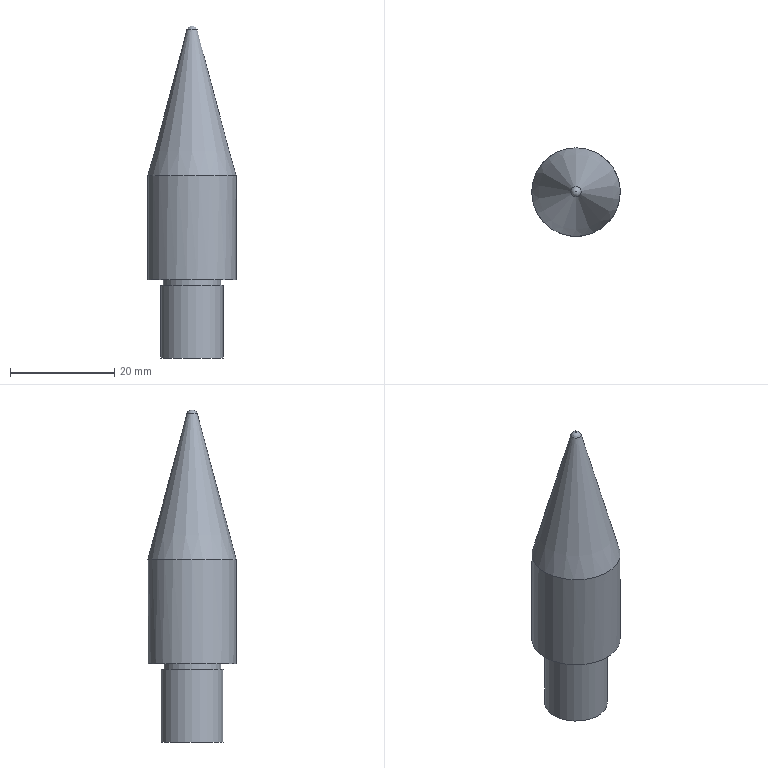Part | NX | features solid 2 | 1 solid | 9 faces | box 17 x 17 x 63.763 mm | volume 8616 mm3 | plane 4 | cylinder 3 | cone 1 | torus 1 | commonest cylinder face diameters 11 x1 12 x1 17 x1
STEP:
#1=CARTESIAN_POINT('',(448.801,-484.613,-19.));
#2=VERTEX_POINT('',#1);
#3=CARTESIAN_POINT('',(457.301,-484.613,-19.));
#4=DIRECTION('',(0.,0.,-1.));
#5=DIRECTION('',(-1.,0.,0.));
#6=AXIS2_PLACEMENT_3D('',#3,#4,#5);
#7=CIRCLE('',#6,8.5);
#8=EDGE_CURVE('',#2,#2,#7,.T.);
#9=ORIENTED_EDGE('',*,*,#8,.T.);
#10=EDGE_LOOP('',(#9));
#11=FACE_BOUND('',#10,.T.);
#12=CARTESIAN_POINT('',(451.801,-484.613,-19.));
#13=VERTEX_POINT('',#12);
#14=CARTESIAN_POINT('',(457.301,-484.613,-19.));
#15=DIRECTION('',(0.,0.,-1.));
#16=DIRECTION('',(-1.,0.,0.));
#17=AXIS2_PLACEMENT_3D('',#14,#15,#16);
#18=CIRCLE('',#17,5.5);
#19=EDGE_CURVE('',#13,#13,#18,.F.);
#20=ORIENTED_EDGE('',*,*,#19,.T.);
#21=EDGE_LOOP('',(#20));
#22=FACE_BOUND('',#21,.T.);
#23=CARTESIAN_POINT('',(457.301,-484.613,-19.));
#24=DIRECTION('',(0.,0.,1.));
#25=DIRECTION('',(-1.,0.,0.));
#26=AXIS2_PLACEMENT_3D('',#23,#24,#25);
#27=PLANE('',#26);
#28=ADVANCED_FACE('',(#11,#22),#27,.F.);
#29=CARTESIAN_POINT('',(457.301,-476.113,1.));
#30=VERTEX_POINT('',#29);
#31=CARTESIAN_POINT('',(457.301,-484.613,1.));
#32=DIRECTION('',(0.,0.,1.));
#33=DIRECTION('',(0.,1.,0.));
#34=AXIS2_PLACEMENT_3D('',#31,#32,#33);
#35=CIRCLE('',#34,8.5);
#36=EDGE_CURVE('',#30,#30,#35,.F.);
#37=ORIENTED_EDGE('',*,*,#36,.T.);
#38=EDGE_LOOP('',(#37));
#39=FACE_BOUND('',#38,.T.);
#40=ORIENTED_EDGE('',*,*,#8,.F.);
#41=EDGE_LOOP('',(#40));
#42=FACE_BOUND('',#41,.T.);
#43=CARTESIAN_POINT('',(457.301,-484.613,-26.556));
#44=DIRECTION('',(0.,0.,1.));
#45=DIRECTION('',(-1.,0.,0.));
#46=AXIS2_PLACEMENT_3D('',#43,#44,#45);
#47=CYLINDRICAL_SURFACE('',#46,8.5);
#48=ADVANCED_FACE('',(#39,#42),#47,.T.);
#49=ORIENTED_EDGE('',*,*,#19,.F.);
#50=EDGE_LOOP('',(#49));
#51=FACE_BOUND('',#50,.T.);
#52=CARTESIAN_POINT('',(451.801,-484.613,-20.));
#53=VERTEX_POINT('',#52);
#54=CARTESIAN_POINT('',(457.301,-484.613,-20.));
#55=DIRECTION('',(0.,0.,-1.));
#56=DIRECTION('',(-1.,0.,0.));
#57=AXIS2_PLACEMENT_3D('',#54,#55,#56);
#58=CIRCLE('',#57,5.5);
#59=EDGE_CURVE('',#53,#53,#58,.T.);
#60=ORIENTED_EDGE('',*,*,#59,.F.);
#61=EDGE_LOOP('',(#60));
#62=FACE_BOUND('',#61,.T.);
#63=CARTESIAN_POINT('',(457.301,-484.613,-16.556));
#64=DIRECTION('',(0.,0.,-1.));
#65=DIRECTION('',(1.,0.,0.));
#66=AXIS2_PLACEMENT_3D('',#63,#64,#65);
#67=CYLINDRICAL_SURFACE('',#66,5.5);
#68=ADVANCED_FACE('',(#51,#62),#67,.T.);
#69=CARTESIAN_POINT('',(451.301,-484.613,-20.));
#70=VERTEX_POINT('',#69);
#71=CARTESIAN_POINT('',(457.301,-484.613,-20.));
#72=DIRECTION('',(0.,0.,-1.));
#73=DIRECTION('',(-1.,0.,0.));
#74=AXIS2_PLACEMENT_3D('',#71,#72,#73);
#75=CIRCLE('',#74,6.);
#76=EDGE_CURVE('',#70,#70,#75,.T.);
#77=ORIENTED_EDGE('',*,*,#76,.F.);
#78=EDGE_LOOP('',(#77));
#79=FACE_BOUND('',#78,.T.);
#80=ORIENTED_EDGE('',*,*,#59,.T.);
#81=EDGE_LOOP('',(#80));
#82=FACE_BOUND('',#81,.T.);
#83=CARTESIAN_POINT('',(457.301,-484.613,-20.));
#84=DIRECTION('',(0.,0.,1.));
#85=DIRECTION('',(-1.,0.,0.));
#86=AXIS2_PLACEMENT_3D('',#83,#84,#85);
#87=PLANE('',#86);
#88=ADVANCED_FACE('',(#79,#82),#87,.T.);
#89=CARTESIAN_POINT('',(451.301,-484.613,-34.));
#90=VERTEX_POINT('',#89);
#91=CARTESIAN_POINT('',(457.301,-484.613,-34.));
#92=DIRECTION('',(0.,0.,-1.));
#93=DIRECTION('',(-1.,0.,0.));
#94=AXIS2_PLACEMENT_3D('',#91,#92,#93);
#95=CIRCLE('',#94,6.);
#96=EDGE_CURVE('',#90,#90,#95,.T.);
#97=ORIENTED_EDGE('',*,*,#96,.F.);
#98=EDGE_LOOP('',(#97));
#99=FACE_BOUND('',#98,.T.);
#100=ORIENTED_EDGE('',*,*,#76,.T.);
#101=EDGE_LOOP('',(#100));
#102=FACE_BOUND('',#101,.T.);
#103=CARTESIAN_POINT('',(457.301,-484.613,-31.556));
#104=DIRECTION('',(0.,0.,1.));
#105=DIRECTION('',(-1.,0.,0.));
#106=AXIS2_PLACEMENT_3D('',#103,#104,#105);
#107=CYLINDRICAL_SURFACE('',#106,6.);
#108=ADVANCED_FACE('',(#99,#102),#107,.T.);
#109=ORIENTED_EDGE('',*,*,#96,.T.);
#110=EDGE_LOOP('',(#109));
#111=FACE_BOUND('',#110,.T.);
#112=CARTESIAN_POINT('',(457.301,-484.613,-34.));
#113=DIRECTION('',(0.,0.,1.));
#114=DIRECTION('',(-1.,0.,0.));
#115=AXIS2_PLACEMENT_3D('',#112,#113,#114);
#116=PLANE('',#115);
#117=ADVANCED_FACE('',(#111),#116,.F.);
#118=CARTESIAN_POINT('',(457.301,-484.588,29.763));
#119=VERTEX_POINT('',#118);
#120=CARTESIAN_POINT('',(457.301,-484.613,29.763));
#121=DIRECTION('',(0.,0.,1.));
#122=DIRECTION('',(0.,1.,0.));
#123=AXIS2_PLACEMENT_3D('',#120,#121,#122);
#124=CIRCLE('',#123,0.02565);
#125=EDGE_CURVE('',#119,#119,#124,.F.);
#126=ORIENTED_EDGE('',*,*,#125,.F.);
#127=EDGE_LOOP('',(#126));
#128=FACE_BOUND('',#127,.T.);
#129=CARTESIAN_POINT('',(459.97,-484.613,29.763));
#130=DIRECTION('',(0.,0.,-1.));
#131=DIRECTION('',(0.,1.,0.));
#132=AXIS2_PLACEMENT_3D('',#129,#130,#131);
#133=PLANE('',#132);
#134=ADVANCED_FACE('',(#128),#133,.F.);
#135=CARTESIAN_POINT('',(457.301,-483.622,29.022));
#136=VERTEX_POINT('',#135);
#137=CARTESIAN_POINT('',(457.301,-484.613,29.022));
#138=DIRECTION('',(0.,0.,1.));
#139=DIRECTION('',(0.,1.,0.));
#140=AXIS2_PLACEMENT_3D('',#137,#138,#139);
#141=CIRCLE('',#140,0.9916);
#142=EDGE_CURVE('',#136,#136,#141,.T.);
#143=ORIENTED_EDGE('',*,*,#142,.F.);
#144=EDGE_LOOP('',(#143));
#145=FACE_BOUND('',#144,.T.);
#146=ORIENTED_EDGE('',*,*,#36,.F.);
#147=EDGE_LOOP('',(#146));
#148=FACE_BOUND('',#147,.T.);
#149=CARTESIAN_POINT('',(457.301,-484.613,22.763));
#150=DIRECTION('',(0.,0.,-1.));
#151=DIRECTION('',(0.,1.,0.));
#152=AXIS2_PLACEMENT_3D('',#149,#150,#151);
#153=CONICAL_SURFACE('',#152,2.669,0.2618);
#154=ADVANCED_FACE('',(#145,#148),#153,.T.);
#155=ORIENTED_EDGE('',*,*,#142,.T.);
#156=EDGE_LOOP('',(#155));
#157=FACE_BOUND('',#156,.T.);
#158=ORIENTED_EDGE('',*,*,#125,.T.);
#159=EDGE_LOOP('',(#158));
#160=FACE_BOUND('',#159,.T.);
#161=CARTESIAN_POINT('',(457.301,-484.613,28.763));
#162=DIRECTION('',(0.,0.,-1.));
#163=DIRECTION('',(0.,1.,0.));
#164=AXIS2_PLACEMENT_3D('',#161,#162,#163);
#165=DEGENERATE_TOROIDAL_SURFACE('',#164,0.02565,1.,.T.);
#166=ADVANCED_FACE('',(#157,#160),#165,.T.);
#167=CLOSED_SHELL('',(#28,#48,#68,#88,#108,#117,#134,#154,#166));
#168=MANIFOLD_SOLID_BREP('',#167);
#169=(LENGTH_UNIT()NAMED_UNIT(*)SI_UNIT(.MILLI.,.METRE.));
#170=UNCERTAINTY_MEASURE_WITH_UNIT(LENGTH_MEASURE(0.00001),#169,'','');
#171=(NAMED_UNIT(*)PLANE_ANGLE_UNIT()SI_UNIT($,.RADIAN.));
#172=(NAMED_UNIT(*)SI_UNIT($,.STERADIAN.)SOLID_ANGLE_UNIT());
#173=(GEOMETRIC_REPRESENTATION_CONTEXT(3)GLOBAL_UNCERTAINTY_ASSIGNED_CONTEXT((#170))GLOBAL_UNIT_ASSIGNED_CONTEXT((#169,#171,#172))REPRESENTATION_CONTEXT('',''));
#174=ADVANCED_BREP_SHAPE_REPRESENTATION('',(#168),#173);